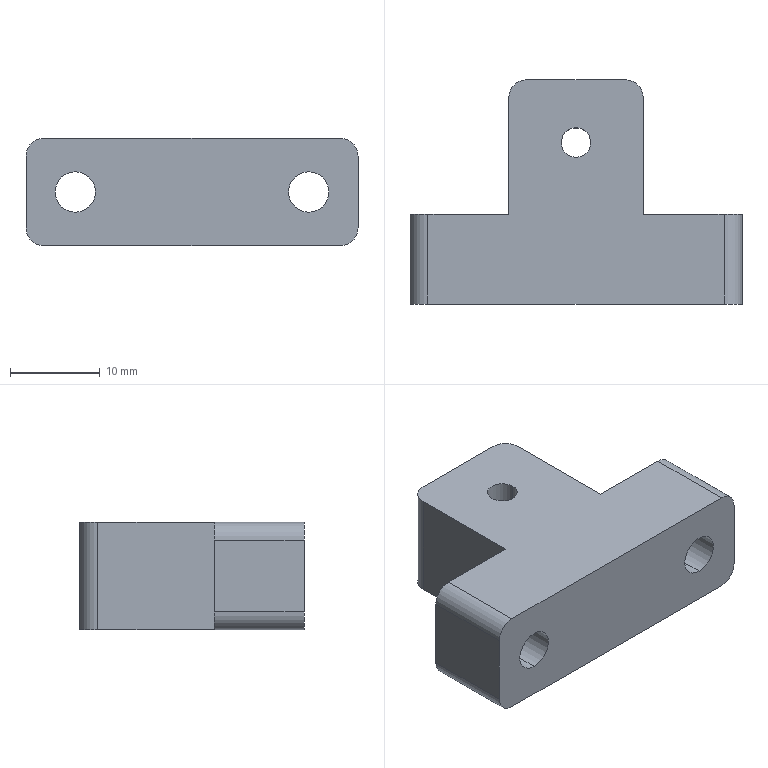Part | NX | features BREP 1 | 1 solid | 28 faces | box 37 x 25 x 12 mm | volume 6187 mm3 | cylinder 16 | plane 12 | commonest cylinder face diameters 4 x6 4.5 x4 9 x4 3.3 x2
STEP:
#1=CARTESIAN_POINT('',(7.5,23.,6.));
#2=VERTEX_POINT('',#1);
#3=CARTESIAN_POINT('',(5.5,25.,6.));
#4=VERTEX_POINT('',#3);
#5=CARTESIAN_POINT('',(5.5,23.,6.));
#6=DIRECTION('',(0.,0.,1.));
#7=DIRECTION('',(-1.,0.,0.));
#8=AXIS2_PLACEMENT_3D('',#5,#6,#7);
#9=CIRCLE('',#8,2.);
#10=EDGE_CURVE('',#2,#4,#9,.T.);
#11=ORIENTED_EDGE('',*,*,#10,.F.);
#12=CARTESIAN_POINT('',(7.5,23.,-6.));
#13=VERTEX_POINT('',#12);
#14=CARTESIAN_POINT('',(7.5,23.,6.));
#15=DIRECTION('',(0.,0.,1.));
#16=VECTOR('',#15,1000.);
#17=LINE('',#14,#16);
#18=EDGE_CURVE('',#13,#2,#17,.T.);
#19=ORIENTED_EDGE('',*,*,#18,.F.);
#20=CARTESIAN_POINT('',(5.5,25.,-6.));
#21=VERTEX_POINT('',#20);
#22=CARTESIAN_POINT('',(5.5,23.,-6.));
#23=DIRECTION('',(0.,0.,-1.));
#24=DIRECTION('',(-1.,0.,0.));
#25=AXIS2_PLACEMENT_3D('',#22,#23,#24);
#26=CIRCLE('',#25,2.);
#27=EDGE_CURVE('',#21,#13,#26,.T.);
#28=ORIENTED_EDGE('',*,*,#27,.F.);
#29=CARTESIAN_POINT('',(5.5,25.,6.));
#30=DIRECTION('',(0.,0.,-1.));
#31=VECTOR('',#30,1000.);
#32=LINE('',#29,#31);
#33=EDGE_CURVE('',#4,#21,#32,.T.);
#34=ORIENTED_EDGE('',*,*,#33,.F.);
#35=EDGE_LOOP('',(#11,#19,#28,#34));
#36=FACE_BOUND('',#35,.T.);
#37=CARTESIAN_POINT('',(5.5,23.,6.));
#38=DIRECTION('',(0.,0.,-1.));
#39=DIRECTION('',(-1.,0.,0.));
#40=AXIS2_PLACEMENT_3D('',#37,#38,#39);
#41=CYLINDRICAL_SURFACE('',#40,2.);
#42=ADVANCED_FACE('',(#36),#41,.T.);
#43=CARTESIAN_POINT('',(-5.5,25.,6.));
#44=VERTEX_POINT('',#43);
#45=CARTESIAN_POINT('',(-7.5,23.,6.));
#46=VERTEX_POINT('',#45);
#47=CARTESIAN_POINT('',(-5.5,23.,6.));
#48=DIRECTION('',(0.,0.,1.));
#49=DIRECTION('',(-1.,0.,0.));
#50=AXIS2_PLACEMENT_3D('',#47,#48,#49);
#51=CIRCLE('',#50,2.);
#52=EDGE_CURVE('',#44,#46,#51,.T.);
#53=ORIENTED_EDGE('',*,*,#52,.F.);
#54=CARTESIAN_POINT('',(-5.5,25.,-6.));
#55=VERTEX_POINT('',#54);
#56=CARTESIAN_POINT('',(-5.5,25.,6.));
#57=DIRECTION('',(0.,0.,1.));
#58=VECTOR('',#57,1000.);
#59=LINE('',#56,#58);
#60=EDGE_CURVE('',#55,#44,#59,.T.);
#61=ORIENTED_EDGE('',*,*,#60,.F.);
#62=CARTESIAN_POINT('',(-7.5,23.,-6.));
#63=VERTEX_POINT('',#62);
#64=CARTESIAN_POINT('',(-5.5,23.,-6.));
#65=DIRECTION('',(0.,0.,-1.));
#66=DIRECTION('',(-1.,0.,0.));
#67=AXIS2_PLACEMENT_3D('',#64,#65,#66);
#68=CIRCLE('',#67,2.);
#69=EDGE_CURVE('',#63,#55,#68,.T.);
#70=ORIENTED_EDGE('',*,*,#69,.F.);
#71=CARTESIAN_POINT('',(-7.5,23.,6.));
#72=DIRECTION('',(0.,0.,-1.));
#73=VECTOR('',#72,1000.);
#74=LINE('',#71,#73);
#75=EDGE_CURVE('',#46,#63,#74,.T.);
#76=ORIENTED_EDGE('',*,*,#75,.F.);
#77=EDGE_LOOP('',(#53,#61,#70,#76));
#78=FACE_BOUND('',#77,.T.);
#79=CARTESIAN_POINT('',(-5.5,23.,6.));
#80=DIRECTION('',(0.,0.,-1.));
#81=DIRECTION('',(-1.,0.,0.));
#82=AXIS2_PLACEMENT_3D('',#79,#80,#81);
#83=CYLINDRICAL_SURFACE('',#82,2.);
#84=ADVANCED_FACE('',(#78),#83,.T.);
#85=CARTESIAN_POINT('',(16.5,0.,-6.));
#86=VERTEX_POINT('',#85);
#87=CARTESIAN_POINT('',(18.5,0.,-4.));
#88=VERTEX_POINT('',#87);
#89=CARTESIAN_POINT('',(16.5,0.,-4.));
#90=DIRECTION('',(0.,-1.,0.));
#91=DIRECTION('',(0.,0.,1.));
#92=AXIS2_PLACEMENT_3D('',#89,#90,#91);
#93=CIRCLE('',#92,2.);
#94=EDGE_CURVE('',#86,#88,#93,.T.);
#95=ORIENTED_EDGE('',*,*,#94,.F.);
#96=CARTESIAN_POINT('',(16.5,10.,-6.));
#97=VERTEX_POINT('',#96);
#98=CARTESIAN_POINT('',(16.5,0.,-6.));
#99=DIRECTION('',(0.,-1.,0.));
#100=VECTOR('',#99,1000.);
#101=LINE('',#98,#100);
#102=EDGE_CURVE('',#97,#86,#101,.T.);
#103=ORIENTED_EDGE('',*,*,#102,.F.);
#104=CARTESIAN_POINT('',(18.5,10.,-4.));
#105=VERTEX_POINT('',#104);
#106=CARTESIAN_POINT('',(16.5,10.,-4.));
#107=DIRECTION('',(0.,1.,0.));
#108=DIRECTION('',(1.,0.,0.));
#109=AXIS2_PLACEMENT_3D('',#106,#107,#108);
#110=CIRCLE('',#109,2.);
#111=EDGE_CURVE('',#105,#97,#110,.T.);
#112=ORIENTED_EDGE('',*,*,#111,.F.);
#113=CARTESIAN_POINT('',(18.5,10.,-4.));
#114=DIRECTION('',(0.,1.,0.));
#115=VECTOR('',#114,1000.);
#116=LINE('',#113,#115);
#117=EDGE_CURVE('',#88,#105,#116,.T.);
#118=ORIENTED_EDGE('',*,*,#117,.F.);
#119=EDGE_LOOP('',(#95,#103,#112,#118));
#120=FACE_BOUND('',#119,.T.);
#121=CARTESIAN_POINT('',(16.5,10.,-4.));
#122=DIRECTION('',(0.,-1.,0.));
#123=DIRECTION('',(1.,0.,0.));
#124=AXIS2_PLACEMENT_3D('',#121,#122,#123);
#125=CYLINDRICAL_SURFACE('',#124,2.);
#126=ADVANCED_FACE('',(#120),#125,.T.);
#127=CARTESIAN_POINT('',(18.5,0.,4.));
#128=VERTEX_POINT('',#127);
#129=CARTESIAN_POINT('',(16.5,0.,6.));
#130=VERTEX_POINT('',#129);
#131=CARTESIAN_POINT('',(16.5,0.,4.));
#132=DIRECTION('',(0.,-1.,0.));
#133=DIRECTION('',(0.,0.,1.));
#134=AXIS2_PLACEMENT_3D('',#131,#132,#133);
#135=CIRCLE('',#134,2.);
#136=EDGE_CURVE('',#128,#130,#135,.T.);
#137=ORIENTED_EDGE('',*,*,#136,.F.);
#138=CARTESIAN_POINT('',(18.5,10.,4.));
#139=VERTEX_POINT('',#138);
#140=CARTESIAN_POINT('',(18.5,10.,4.));
#141=DIRECTION('',(0.,-1.,0.));
#142=VECTOR('',#141,1000.);
#143=LINE('',#140,#142);
#144=EDGE_CURVE('',#139,#128,#143,.T.);
#145=ORIENTED_EDGE('',*,*,#144,.F.);
#146=CARTESIAN_POINT('',(16.5,10.,6.));
#147=VERTEX_POINT('',#146);
#148=CARTESIAN_POINT('',(16.5,10.,4.));
#149=DIRECTION('',(0.,1.,0.));
#150=DIRECTION('',(1.,0.,0.));
#151=AXIS2_PLACEMENT_3D('',#148,#149,#150);
#152=CIRCLE('',#151,2.);
#153=EDGE_CURVE('',#147,#139,#152,.T.);
#154=ORIENTED_EDGE('',*,*,#153,.F.);
#155=CARTESIAN_POINT('',(16.5,0.,6.));
#156=DIRECTION('',(0.,1.,0.));
#157=VECTOR('',#156,1000.);
#158=LINE('',#155,#157);
#159=EDGE_CURVE('',#130,#147,#158,.T.);
#160=ORIENTED_EDGE('',*,*,#159,.F.);
#161=EDGE_LOOP('',(#137,#145,#154,#160));
#162=FACE_BOUND('',#161,.T.);
#163=CARTESIAN_POINT('',(16.5,0.,4.));
#164=DIRECTION('',(0.,1.,0.));
#165=DIRECTION('',(-1.,0.,0.));
#166=AXIS2_PLACEMENT_3D('',#163,#164,#165);
#167=CYLINDRICAL_SURFACE('',#166,2.);
#168=ADVANCED_FACE('',(#162),#167,.T.);
#169=CARTESIAN_POINT('',(-16.5,10.,-6.));
#170=VERTEX_POINT('',#169);
#171=CARTESIAN_POINT('',(-18.5,10.,-4.));
#172=VERTEX_POINT('',#171);
#173=CARTESIAN_POINT('',(-16.5,10.,-4.));
#174=DIRECTION('',(0.,1.,0.));
#175=DIRECTION('',(1.,0.,0.));
#176=AXIS2_PLACEMENT_3D('',#173,#174,#175);
#177=CIRCLE('',#176,2.);
#178=EDGE_CURVE('',#170,#172,#177,.T.);
#179=ORIENTED_EDGE('',*,*,#178,.F.);
#180=CARTESIAN_POINT('',(-16.5,0.,-6.));
#181=VERTEX_POINT('',#180);
#182=CARTESIAN_POINT('',(-16.5,10.,-6.));
#183=DIRECTION('',(0.,1.,0.));
#184=VECTOR('',#183,1000.);
#185=LINE('',#182,#184);
#186=EDGE_CURVE('',#181,#170,#185,.T.);
#187=ORIENTED_EDGE('',*,*,#186,.F.);
#188=CARTESIAN_POINT('',(-18.5,0.,-4.));
#189=VERTEX_POINT('',#188);
#190=CARTESIAN_POINT('',(-16.5,0.,-4.));
#191=DIRECTION('',(0.,-1.,0.));
#192=DIRECTION('',(0.,0.,1.));
#193=AXIS2_PLACEMENT_3D('',#190,#191,#192);
#194=CIRCLE('',#193,2.);
#195=EDGE_CURVE('',#189,#181,#194,.T.);
#196=ORIENTED_EDGE('',*,*,#195,.F.);
#197=CARTESIAN_POINT('',(-18.5,0.,-4.));
#198=DIRECTION('',(0.,-1.,0.));
#199=VECTOR('',#198,1000.);
#200=LINE('',#197,#199);
#201=EDGE_CURVE('',#172,#189,#200,.T.);
#202=ORIENTED_EDGE('',*,*,#201,.F.);
#203=EDGE_LOOP('',(#179,#187,#196,#202));
#204=FACE_BOUND('',#203,.T.);
#205=CARTESIAN_POINT('',(-16.5,10.,-4.));
#206=DIRECTION('',(0.,1.,0.));
#207=DIRECTION('',(-1.,0.,0.));
#208=AXIS2_PLACEMENT_3D('',#205,#206,#207);
#209=CYLINDRICAL_SURFACE('',#208,2.);
#210=ADVANCED_FACE('',(#204),#209,.T.);
#211=CARTESIAN_POINT('',(-18.5,10.,4.));
#212=VERTEX_POINT('',#211);
#213=CARTESIAN_POINT('',(-16.5,10.,6.));
#214=VERTEX_POINT('',#213);
#215=CARTESIAN_POINT('',(-16.5,10.,4.));
#216=DIRECTION('',(0.,1.,0.));
#217=DIRECTION('',(1.,0.,0.));
#218=AXIS2_PLACEMENT_3D('',#215,#216,#217);
#219=CIRCLE('',#218,2.);
#220=EDGE_CURVE('',#212,#214,#219,.T.);
#221=ORIENTED_EDGE('',*,*,#220,.F.);
#222=CARTESIAN_POINT('',(-18.5,0.,4.));
#223=VERTEX_POINT('',#222);
#224=CARTESIAN_POINT('',(-18.5,10.,4.));
#225=DIRECTION('',(0.,1.,0.));
#226=VECTOR('',#225,1000.);
#227=LINE('',#224,#226);
#228=EDGE_CURVE('',#223,#212,#227,.T.);
#229=ORIENTED_EDGE('',*,*,#228,.F.);
#230=CARTESIAN_POINT('',(-16.5,0.,6.));
#231=VERTEX_POINT('',#230);
#232=CARTESIAN_POINT('',(-16.5,0.,4.));
#233=DIRECTION('',(0.,-1.,0.));
#234=DIRECTION('',(0.,0.,1.));
#235=AXIS2_PLACEMENT_3D('',#232,#233,#234);
#236=CIRCLE('',#235,2.);
#237=EDGE_CURVE('',#231,#223,#236,.T.);
#238=ORIENTED_EDGE('',*,*,#237,.F.);
#239=CARTESIAN_POINT('',(-16.5,0.,6.));
#240=DIRECTION('',(0.,-1.,0.));
#241=VECTOR('',#240,1000.);
#242=LINE('',#239,#241);
#243=EDGE_CURVE('',#214,#231,#242,.T.);
#244=ORIENTED_EDGE('',*,*,#243,.F.);
#245=EDGE_LOOP('',(#221,#229,#238,#244));
#246=FACE_BOUND('',#245,.T.);
#247=CARTESIAN_POINT('',(-16.5,0.,4.));
#248=DIRECTION('',(0.,-1.,0.));
#249=DIRECTION('',(1.,0.,0.));
#250=AXIS2_PLACEMENT_3D('',#247,#248,#249);
#251=CYLINDRICAL_SURFACE('',#250,2.);
#252=ADVANCED_FACE('',(#246),#251,.T.);
#253=CARTESIAN_POINT('',(-1.65,18.,6.));
#254=VERTEX_POINT('',#253);
#255=CARTESIAN_POINT('',(-1.65,18.,-6.));
#256=VERTEX_POINT('',#255);
#257=CARTESIAN_POINT('',(-1.65,18.,6.));
#258=DIRECTION('',(0.,0.,1.));
#259=VECTOR('',#258,1000.);
#260=LINE('',#257,#259);
#261=EDGE_CURVE('',#254,#256,#260,.F.);
#262=ORIENTED_EDGE('',*,*,#261,.T.);
#263=CARTESIAN_POINT('',(1.65,18.,-6.));
#264=VERTEX_POINT('',#263);
#265=CARTESIAN_POINT('',(0.,18.,-6.));
#266=DIRECTION('',(0.,0.,-1.));
#267=DIRECTION('',(-1.,0.,0.));
#268=AXIS2_PLACEMENT_3D('',#265,#266,#267);
#269=CIRCLE('',#268,1.65);
#270=EDGE_CURVE('',#256,#264,#269,.T.);
#271=ORIENTED_EDGE('',*,*,#270,.T.);
#272=CARTESIAN_POINT('',(1.65,18.,6.));
#273=VERTEX_POINT('',#272);
#274=CARTESIAN_POINT('',(1.65,18.,6.));
#275=DIRECTION('',(0.,0.,1.));
#276=VECTOR('',#275,1000.);
#277=LINE('',#274,#276);
#278=EDGE_CURVE('',#273,#264,#277,.F.);
#279=ORIENTED_EDGE('',*,*,#278,.F.);
#280=CARTESIAN_POINT('',(0.,18.,6.));
#281=DIRECTION('',(0.,0.,1.));
#282=DIRECTION('',(1.,0.,0.));
#283=AXIS2_PLACEMENT_3D('',#280,#281,#282);
#284=CIRCLE('',#283,1.65);
#285=EDGE_CURVE('',#273,#254,#284,.T.);
#286=ORIENTED_EDGE('',*,*,#285,.T.);
#287=EDGE_LOOP('',(#262,#271,#279,#286));
#288=FACE_BOUND('',#287,.T.);
#289=CARTESIAN_POINT('',(0.,18.,6.));
#290=DIRECTION('',(0.,0.,1.));
#291=DIRECTION('',(1.,0.,0.));
#292=AXIS2_PLACEMENT_3D('',#289,#290,#291);
#293=CYLINDRICAL_SURFACE('',#292,1.65);
#294=ADVANCED_FACE('',(#288),#293,.F.);
#295=CARTESIAN_POINT('',(13.,10.,-4.5));
#296=VERTEX_POINT('',#295);
#297=CARTESIAN_POINT('',(13.,5.,-4.5));
#298=VERTEX_POINT('',#297);
#299=CARTESIAN_POINT('',(13.,10.,-4.5));
#300=DIRECTION('',(0.,1.,0.));
#301=VECTOR('',#300,1000.);
#302=LINE('',#299,#301);
#303=EDGE_CURVE('',#296,#298,#302,.F.);
#304=ORIENTED_EDGE('',*,*,#303,.T.);
#305=CARTESIAN_POINT('',(13.,5.,4.5));
#306=VERTEX_POINT('',#305);
#307=CARTESIAN_POINT('',(13.,5.,0.));
#308=DIRECTION('',(0.,1.,0.));
#309=DIRECTION('',(0.,0.,1.));
#310=AXIS2_PLACEMENT_3D('',#307,#308,#309);
#311=CIRCLE('',#310,4.5);
#312=EDGE_CURVE('',#306,#298,#311,.T.);
#313=ORIENTED_EDGE('',*,*,#312,.F.);
#314=CARTESIAN_POINT('',(13.,10.,4.5));
#315=VERTEX_POINT('',#314);
#316=CARTESIAN_POINT('',(13.,10.,4.5));
#317=DIRECTION('',(0.,1.,0.));
#318=VECTOR('',#317,1000.);
#319=LINE('',#316,#318);
#320=EDGE_CURVE('',#315,#306,#319,.F.);
#321=ORIENTED_EDGE('',*,*,#320,.F.);
#322=CARTESIAN_POINT('',(13.,10.,0.));
#323=DIRECTION('',(0.,1.,0.));
#324=DIRECTION('',(0.,0.,1.));
#325=AXIS2_PLACEMENT_3D('',#322,#323,#324);
#326=CIRCLE('',#325,4.5);
#327=EDGE_CURVE('',#315,#296,#326,.T.);
#328=ORIENTED_EDGE('',*,*,#327,.T.);
#329=EDGE_LOOP('',(#304,#313,#321,#328));
#330=FACE_BOUND('',#329,.T.);
#331=CARTESIAN_POINT('',(13.,10.,0.));
#332=DIRECTION('',(0.,1.,0.));
#333=DIRECTION('',(0.,0.,1.));
#334=AXIS2_PLACEMENT_3D('',#331,#332,#333);
#335=CYLINDRICAL_SURFACE('',#334,4.5);
#336=ADVANCED_FACE('',(#330),#335,.F.);
#337=ORIENTED_EDGE('',*,*,#312,.T.);
#338=CARTESIAN_POINT('',(13.,5.,0.));
#339=DIRECTION('',(0.,1.,0.));
#340=DIRECTION('',(0.,0.,1.));
#341=AXIS2_PLACEMENT_3D('',#338,#339,#340);
#342=CIRCLE('',#341,4.5);
#343=EDGE_CURVE('',#298,#306,#342,.T.);
#344=ORIENTED_EDGE('',*,*,#343,.T.);
#345=EDGE_LOOP('',(#337,#344));
#346=FACE_BOUND('',#345,.T.);
#347=CARTESIAN_POINT('',(13.,5.,2.25));
#348=VERTEX_POINT('',#347);
#349=CARTESIAN_POINT('',(13.,5.,-2.25));
#350=VERTEX_POINT('',#349);
#351=CARTESIAN_POINT('',(13.,5.,0.));
#352=DIRECTION('',(0.,1.,0.));
#353=DIRECTION('',(0.,0.,1.));
#354=AXIS2_PLACEMENT_3D('',#351,#352,#353);
#355=CIRCLE('',#354,2.25);
#356=EDGE_CURVE('',#348,#350,#355,.T.);
#357=ORIENTED_EDGE('',*,*,#356,.F.);
#358=CARTESIAN_POINT('',(13.,5.,0.));
#359=DIRECTION('',(0.,1.,0.));
#360=DIRECTION('',(0.,0.,1.));
#361=AXIS2_PLACEMENT_3D('',#358,#359,#360);
#362=CIRCLE('',#361,2.25);
#363=EDGE_CURVE('',#350,#348,#362,.T.);
#364=ORIENTED_EDGE('',*,*,#363,.F.);
#365=EDGE_LOOP('',(#357,#364));
#366=FACE_BOUND('',#365,.T.);
#367=CARTESIAN_POINT('',(15.25,5.,0.));
#368=DIRECTION('',(0.,-1.,0.));
#369=DIRECTION('',(0.,0.,-1.));
#370=AXIS2_PLACEMENT_3D('',#367,#368,#369);
#371=PLANE('',#370);
#372=ADVANCED_FACE('',(#346,#366),#371,.F.);
#373=CARTESIAN_POINT('',(13.,0.,-2.25));
#374=VERTEX_POINT('',#373);
#375=CARTESIAN_POINT('',(13.,10.,-2.25));
#376=DIRECTION('',(0.,1.,0.));
#377=VECTOR('',#376,1000.);
#378=LINE('',#375,#377);
#379=EDGE_CURVE('',#350,#374,#378,.F.);
#380=ORIENTED_EDGE('',*,*,#379,.T.);
#381=CARTESIAN_POINT('',(13.,0.,2.25));
#382=VERTEX_POINT('',#381);
#383=CARTESIAN_POINT('',(13.,0.,0.));
#384=DIRECTION('',(0.,1.,0.));
#385=DIRECTION('',(0.,0.,1.));
#386=AXIS2_PLACEMENT_3D('',#383,#384,#385);
#387=CIRCLE('',#386,2.25);
#388=EDGE_CURVE('',#382,#374,#387,.T.);
#389=ORIENTED_EDGE('',*,*,#388,.F.);
#390=CARTESIAN_POINT('',(13.,10.,2.25));
#391=DIRECTION('',(0.,1.,0.));
#392=VECTOR('',#391,1000.);
#393=LINE('',#390,#392);
#394=EDGE_CURVE('',#348,#382,#393,.F.);
#395=ORIENTED_EDGE('',*,*,#394,.F.);
#396=ORIENTED_EDGE('',*,*,#356,.T.);
#397=EDGE_LOOP('',(#380,#389,#395,#396));
#398=FACE_BOUND('',#397,.T.);
#399=CARTESIAN_POINT('',(13.,10.,0.));
#400=DIRECTION('',(0.,1.,0.));
#401=DIRECTION('',(0.,0.,1.));
#402=AXIS2_PLACEMENT_3D('',#399,#400,#401);
#403=CYLINDRICAL_SURFACE('',#402,2.25);
#404=ADVANCED_FACE('',(#398),#403,.F.);
#405=CARTESIAN_POINT('',(-13.,10.,-4.5));
#406=VERTEX_POINT('',#405);
#407=CARTESIAN_POINT('',(-13.,5.,-4.5));
#408=VERTEX_POINT('',#407);
#409=CARTESIAN_POINT('',(-13.,10.,-4.5));
#410=DIRECTION('',(0.,1.,0.));
#411=VECTOR('',#410,1000.);
#412=LINE('',#409,#411);
#413=EDGE_CURVE('',#406,#408,#412,.F.);
#414=ORIENTED_EDGE('',*,*,#413,.T.);
#415=CARTESIAN_POINT('',(-13.,5.,4.5));
#416=VERTEX_POINT('',#415);
#417=CARTESIAN_POINT('',(-13.,5.,0.));
#418=DIRECTION('',(0.,1.,0.));
#419=DIRECTION('',(0.,0.,1.));
#420=AXIS2_PLACEMENT_3D('',#417,#418,#419);
#421=CIRCLE('',#420,4.5);
#422=EDGE_CURVE('',#416,#408,#421,.T.);
#423=ORIENTED_EDGE('',*,*,#422,.F.);
#424=CARTESIAN_POINT('',(-13.,10.,4.5));
#425=VERTEX_POINT('',#424);
#426=CARTESIAN_POINT('',(-13.,10.,4.5));
#427=DIRECTION('',(0.,1.,0.));
#428=VECTOR('',#427,1000.);
#429=LINE('',#426,#428);
#430=EDGE_CURVE('',#425,#416,#429,.F.);
#431=ORIENTED_EDGE('',*,*,#430,.F.);
#432=CARTESIAN_POINT('',(-13.,10.,0.));
#433=DIRECTION('',(0.,1.,0.));
#434=DIRECTION('',(0.,0.,1.));
#435=AXIS2_PLACEMENT_3D('',#432,#433,#434);
#436=CIRCLE('',#435,4.5);
#437=EDGE_CURVE('',#425,#406,#436,.T.);
#438=ORIENTED_EDGE('',*,*,#437,.T.);
#439=EDGE_LOOP('',(#414,#423,#431,#438));
#440=FACE_BOUND('',#439,.T.);
#441=CARTESIAN_POINT('',(-13.,10.,0.));
#442=DIRECTION('',(0.,1.,0.));
#443=DIRECTION('',(0.,0.,1.));
#444=AXIS2_PLACEMENT_3D('',#441,#442,#443);
#445=CYLINDRICAL_SURFACE('',#444,4.5);
#446=ADVANCED_FACE('',(#440),#445,.F.);
#447=ORIENTED_EDGE('',*,*,#422,.T.);
#448=CARTESIAN_POINT('',(-13.,5.,0.));
#449=DIRECTION('',(0.,1.,0.));
#450=DIRECTION('',(0.,0.,1.));
#451=AXIS2_PLACEMENT_3D('',#448,#449,#450);
#452=CIRCLE('',#451,4.5);
#453=EDGE_CURVE('',#408,#416,#452,.T.);
#454=ORIENTED_EDGE('',*,*,#453,.T.);
#455=EDGE_LOOP('',(#447,#454));
#456=FACE_BOUND('',#455,.T.);
#457=CARTESIAN_POINT('',(-13.,5.,2.25));
#458=VERTEX_POINT('',#457);
#459=CARTESIAN_POINT('',(-13.,5.,-2.25));
#460=VERTEX_POINT('',#459);
#461=CARTESIAN_POINT('',(-13.,5.,0.));
#462=DIRECTION('',(0.,1.,0.));
#463=DIRECTION('',(0.,0.,1.));
#464=AXIS2_PLACEMENT_3D('',#461,#462,#463);
#465=CIRCLE('',#464,2.25);
#466=EDGE_CURVE('',#458,#460,#465,.T.);
#467=ORIENTED_EDGE('',*,*,#466,.F.);
#468=CARTESIAN_POINT('',(-13.,5.,0.));
#469=DIRECTION('',(0.,1.,0.));
#470=DIRECTION('',(0.,0.,1.));
#471=AXIS2_PLACEMENT_3D('',#468,#469,#470);
#472=CIRCLE('',#471,2.25);
#473=EDGE_CURVE('',#460,#458,#472,.T.);
#474=ORIENTED_EDGE('',*,*,#473,.F.);
#475=EDGE_LOOP('',(#467,#474));
#476=FACE_BOUND('',#475,.T.);
#477=CARTESIAN_POINT('',(-10.75,5.,0.));
#478=DIRECTION('',(0.,-1.,0.));
#479=DIRECTION('',(0.,0.,-1.));
#480=AXIS2_PLACEMENT_3D('',#477,#478,#479);
#481=PLANE('',#480);
#482=ADVANCED_FACE('',(#456,#476),#481,.F.);
#483=CARTESIAN_POINT('',(-13.,0.,-2.25));
#484=VERTEX_POINT('',#483);
#485=CARTESIAN_POINT('',(-13.,10.,-2.25));
#486=DIRECTION('',(0.,1.,0.));
#487=VECTOR('',#486,1000.);
#488=LINE('',#485,#487);
#489=EDGE_CURVE('',#460,#484,#488,.F.);
#490=ORIENTED_EDGE('',*,*,#489,.T.);
#491=CARTESIAN_POINT('',(-13.,0.,2.25));
#492=VERTEX_POINT('',#491);
#493=CARTESIAN_POINT('',(-13.,0.,0.));
#494=DIRECTION('',(0.,1.,0.));
#495=DIRECTION('',(0.,0.,1.));
#496=AXIS2_PLACEMENT_3D('',#493,#494,#495);
#497=CIRCLE('',#496,2.25);
#498=EDGE_CURVE('',#492,#484,#497,.T.);
#499=ORIENTED_EDGE('',*,*,#498,.F.);
#500=CARTESIAN_POINT('',(-13.,10.,2.25));
#501=DIRECTION('',(0.,1.,0.));
#502=VECTOR('',#501,1000.);
#503=LINE('',#500,#502);
#504=EDGE_CURVE('',#458,#492,#503,.F.);
#505=ORIENTED_EDGE('',*,*,#504,.F.);
#506=ORIENTED_EDGE('',*,*,#466,.T.);
#507=EDGE_LOOP('',(#490,#499,#505,#506));
#508=FACE_BOUND('',#507,.T.);
#509=CARTESIAN_POINT('',(-13.,10.,0.));
#510=DIRECTION('',(0.,1.,0.));
#511=DIRECTION('',(0.,0.,1.));
#512=AXIS2_PLACEMENT_3D('',#509,#510,#511);
#513=CYLINDRICAL_SURFACE('',#512,2.25);
#514=ADVANCED_FACE('',(#508),#513,.F.);
#515=CARTESIAN_POINT('',(-18.5,0.,-6.));
#516=DIRECTION('',(1.,0.,0.));
#517=VECTOR('',#516,1000.);
#518=LINE('',#515,#517);
#519=EDGE_CURVE('',#181,#86,#518,.T.);
#520=ORIENTED_EDGE('',*,*,#519,.F.);
#521=ORIENTED_EDGE('',*,*,#186,.T.);
#522=CARTESIAN_POINT('',(-7.5,10.,-6.));
#523=VERTEX_POINT('',#522);
#524=CARTESIAN_POINT('',(-7.5,10.,-6.));
#525=DIRECTION('',(-1.,0.,0.));
#526=VECTOR('',#525,1000.);
#527=LINE('',#524,#526);
#528=EDGE_CURVE('',#523,#170,#527,.T.);
#529=ORIENTED_EDGE('',*,*,#528,.F.);
#530=CARTESIAN_POINT('',(-7.5,25.,-6.));
#531=DIRECTION('',(0.,-1.,0.));
#532=VECTOR('',#531,1000.);
#533=LINE('',#530,#532);
#534=EDGE_CURVE('',#63,#523,#533,.T.);
#535=ORIENTED_EDGE('',*,*,#534,.F.);
#536=ORIENTED_EDGE('',*,*,#69,.T.);
#537=CARTESIAN_POINT('',(7.5,25.,-6.));
#538=DIRECTION('',(-1.,0.,0.));
#539=VECTOR('',#538,1000.);
#540=LINE('',#537,#539);
#541=EDGE_CURVE('',#21,#55,#540,.T.);
#542=ORIENTED_EDGE('',*,*,#541,.F.);
#543=ORIENTED_EDGE('',*,*,#27,.T.);
#544=CARTESIAN_POINT('',(7.5,10.,-6.));
#545=VERTEX_POINT('',#544);
#546=CARTESIAN_POINT('',(7.5,25.,-6.));
#547=DIRECTION('',(0.,1.,0.));
#548=VECTOR('',#547,1000.);
#549=LINE('',#546,#548);
#550=EDGE_CURVE('',#545,#13,#549,.T.);
#551=ORIENTED_EDGE('',*,*,#550,.F.);
#552=CARTESIAN_POINT('',(7.5,10.,-6.));
#553=DIRECTION('',(-1.,0.,0.));
#554=VECTOR('',#553,1000.);
#555=LINE('',#552,#554);
#556=EDGE_CURVE('',#97,#545,#555,.T.);
#557=ORIENTED_EDGE('',*,*,#556,.F.);
#558=ORIENTED_EDGE('',*,*,#102,.T.);
#559=EDGE_LOOP('',(#520,#521,#529,#535,#536,#542,#543,#551,#557,#558));
#560=FACE_BOUND('',#559,.T.);
#561=CARTESIAN_POINT('',(0.,18.,-6.));
#562=DIRECTION('',(0.,0.,-1.));
#563=DIRECTION('',(-1.,0.,0.));
#564=AXIS2_PLACEMENT_3D('',#561,#562,#563);
#565=CIRCLE('',#564,1.65);
#566=EDGE_CURVE('',#264,#256,#565,.T.);
#567=ORIENTED_EDGE('',*,*,#566,.F.);
#568=ORIENTED_EDGE('',*,*,#270,.F.);
#569=EDGE_LOOP('',(#567,#568));
#570=FACE_BOUND('',#569,.T.);
#571=CARTESIAN_POINT('',(0.,0.,-6.));
#572=DIRECTION('',(0.,0.,-1.));
#573=DIRECTION('',(-1.,0.,0.));
#574=AXIS2_PLACEMENT_3D('',#571,#572,#573);
#575=PLANE('',#574);
#576=ADVANCED_FACE('',(#560,#570),#575,.T.);
#577=CARTESIAN_POINT('',(-7.5,10.,6.));
#578=VERTEX_POINT('',#577);
#579=CARTESIAN_POINT('',(-7.5,10.,6.));
#580=DIRECTION('',(-1.,0.,0.));
#581=VECTOR('',#580,1000.);
#582=LINE('',#579,#581);
#583=EDGE_CURVE('',#578,#214,#582,.T.);
#584=ORIENTED_EDGE('',*,*,#583,.T.);
#585=ORIENTED_EDGE('',*,*,#243,.T.);
#586=CARTESIAN_POINT('',(-18.5,0.,6.));
#587=DIRECTION('',(1.,0.,0.));
#588=VECTOR('',#587,1000.);
#589=LINE('',#586,#588);
#590=EDGE_CURVE('',#231,#130,#589,.T.);
#591=ORIENTED_EDGE('',*,*,#590,.T.);
#592=ORIENTED_EDGE('',*,*,#159,.T.);
#593=CARTESIAN_POINT('',(7.5,10.,6.));
#594=VERTEX_POINT('',#593);
#595=CARTESIAN_POINT('',(7.5,10.,6.));
#596=DIRECTION('',(-1.,0.,0.));
#597=VECTOR('',#596,1000.);
#598=LINE('',#595,#597);
#599=EDGE_CURVE('',#147,#594,#598,.T.);
#600=ORIENTED_EDGE('',*,*,#599,.T.);
#601=CARTESIAN_POINT('',(7.5,25.,6.));
#602=DIRECTION('',(0.,1.,0.));
#603=VECTOR('',#602,1000.);
#604=LINE('',#601,#603);
#605=EDGE_CURVE('',#594,#2,#604,.T.);
#606=ORIENTED_EDGE('',*,*,#605,.T.);
#607=ORIENTED_EDGE('',*,*,#10,.T.);
#608=CARTESIAN_POINT('',(7.5,25.,6.));
#609=DIRECTION('',(-1.,0.,0.));
#610=VECTOR('',#609,1000.);
#611=LINE('',#608,#610);
#612=EDGE_CURVE('',#4,#44,#611,.T.);
#613=ORIENTED_EDGE('',*,*,#612,.T.);
#614=ORIENTED_EDGE('',*,*,#52,.T.);
#615=CARTESIAN_POINT('',(-7.5,25.,6.));
#616=DIRECTION('',(0.,-1.,0.));
#617=VECTOR('',#616,1000.);
#618=LINE('',#615,#617);
#619=EDGE_CURVE('',#46,#578,#618,.T.);
#620=ORIENTED_EDGE('',*,*,#619,.T.);
#621=EDGE_LOOP('',(#584,#585,#591,#592,#600,#606,#607,#613,#614,#620));
#622=FACE_BOUND('',#621,.T.);
#623=ORIENTED_EDGE('',*,*,#285,.F.);
#624=CARTESIAN_POINT('',(0.,18.,6.));
#625=DIRECTION('',(0.,0.,1.));
#626=DIRECTION('',(1.,0.,0.));
#627=AXIS2_PLACEMENT_3D('',#624,#625,#626);
#628=CIRCLE('',#627,1.65);
#629=EDGE_CURVE('',#254,#273,#628,.T.);
#630=ORIENTED_EDGE('',*,*,#629,.F.);
#631=EDGE_LOOP('',(#623,#630));
#632=FACE_BOUND('',#631,.T.);
#633=CARTESIAN_POINT('',(0.,0.,6.));
#634=DIRECTION('',(0.,0.,-1.));
#635=DIRECTION('',(-1.,0.,0.));
#636=AXIS2_PLACEMENT_3D('',#633,#634,#635);
#637=PLANE('',#636);
#638=ADVANCED_FACE('',(#622,#632),#637,.F.);
#639=ORIENTED_EDGE('',*,*,#541,.T.);
#640=ORIENTED_EDGE('',*,*,#60,.T.);
#641=ORIENTED_EDGE('',*,*,#612,.F.);
#642=ORIENTED_EDGE('',*,*,#33,.T.);
#643=EDGE_LOOP('',(#639,#640,#641,#642));
#644=FACE_BOUND('',#643,.T.);
#645=CARTESIAN_POINT('',(7.5,25.,6.));
#646=DIRECTION('',(0.,-1.,0.));
#647=DIRECTION('',(0.,0.,-1.));
#648=AXIS2_PLACEMENT_3D('',#645,#646,#647);
#649=PLANE('',#648);
#650=ADVANCED_FACE('',(#644),#649,.F.);
#651=ORIENTED_EDGE('',*,*,#550,.T.);
#652=ORIENTED_EDGE('',*,*,#18,.T.);
#653=ORIENTED_EDGE('',*,*,#605,.F.);
#654=CARTESIAN_POINT('',(7.5,10.,6.));
#655=DIRECTION('',(0.,0.,-1.));
#656=VECTOR('',#655,1000.);
#657=LINE('',#654,#656);
#658=EDGE_CURVE('',#594,#545,#657,.T.);
#659=ORIENTED_EDGE('',*,*,#658,.T.);
#660=EDGE_LOOP('',(#651,#652,#653,#659));
#661=FACE_BOUND('',#660,.T.);
#662=CARTESIAN_POINT('',(7.5,25.,6.));
#663=DIRECTION('',(-1.,0.,0.));
#664=DIRECTION('',(0.,-1.,0.));
#665=AXIS2_PLACEMENT_3D('',#662,#663,#664);
#666=PLANE('',#665);
#667=ADVANCED_FACE('',(#661),#666,.F.);
#668=CARTESIAN_POINT('',(18.5,10.,6.));
#669=DIRECTION('',(0.,0.,-1.));
#670=VECTOR('',#669,1000.);
#671=LINE('',#668,#670);
#672=EDGE_CURVE('',#139,#105,#671,.T.);
#673=ORIENTED_EDGE('',*,*,#672,.F.);
#674=ORIENTED_EDGE('',*,*,#144,.T.);
#675=CARTESIAN_POINT('',(18.5,0.,6.));
#676=DIRECTION('',(0.,0.,-1.));
#677=VECTOR('',#676,1000.);
#678=LINE('',#675,#677);
#679=EDGE_CURVE('',#128,#88,#678,.T.);
#680=ORIENTED_EDGE('',*,*,#679,.T.);
#681=ORIENTED_EDGE('',*,*,#117,.T.);
#682=EDGE_LOOP('',(#673,#674,#680,#681));
#683=FACE_BOUND('',#682,.T.);
#684=CARTESIAN_POINT('',(18.5,10.,6.));
#685=DIRECTION('',(-1.,0.,0.));
#686=DIRECTION('',(0.,-1.,0.));
#687=AXIS2_PLACEMENT_3D('',#684,#685,#686);
#688=PLANE('',#687);
#689=ADVANCED_FACE('',(#683),#688,.F.);
#690=ORIENTED_EDGE('',*,*,#590,.F.);
#691=ORIENTED_EDGE('',*,*,#237,.T.);
#692=CARTESIAN_POINT('',(-18.5,0.,6.));
#693=DIRECTION('',(0.,0.,-1.));
#694=VECTOR('',#693,1000.);
#695=LINE('',#692,#694);
#696=EDGE_CURVE('',#223,#189,#695,.T.);
#697=ORIENTED_EDGE('',*,*,#696,.T.);
#698=ORIENTED_EDGE('',*,*,#195,.T.);
#699=ORIENTED_EDGE('',*,*,#519,.T.);
#700=ORIENTED_EDGE('',*,*,#94,.T.);
#701=ORIENTED_EDGE('',*,*,#679,.F.);
#702=ORIENTED_EDGE('',*,*,#136,.T.);
#703=EDGE_LOOP('',(#690,#691,#697,#698,#699,#700,#701,#702));
#704=FACE_BOUND('',#703,.T.);
#705=ORIENTED_EDGE('',*,*,#498,.T.);
#706=CARTESIAN_POINT('',(-13.,0.,0.));
#707=DIRECTION('',(0.,1.,0.));
#708=DIRECTION('',(0.,0.,1.));
#709=AXIS2_PLACEMENT_3D('',#706,#707,#708);
#710=CIRCLE('',#709,2.25);
#711=EDGE_CURVE('',#484,#492,#710,.T.);
#712=ORIENTED_EDGE('',*,*,#711,.T.);
#713=EDGE_LOOP('',(#705,#712));
#714=FACE_BOUND('',#713,.T.);
#715=ORIENTED_EDGE('',*,*,#388,.T.);
#716=CARTESIAN_POINT('',(13.,0.,0.));
#717=DIRECTION('',(0.,1.,0.));
#718=DIRECTION('',(0.,0.,1.));
#719=AXIS2_PLACEMENT_3D('',#716,#717,#718);
#720=CIRCLE('',#719,2.25);
#721=EDGE_CURVE('',#374,#382,#720,.T.);
#722=ORIENTED_EDGE('',*,*,#721,.T.);
#723=EDGE_LOOP('',(#715,#722));
#724=FACE_BOUND('',#723,.T.);
#725=CARTESIAN_POINT('',(-18.5,0.,6.));
#726=DIRECTION('',(0.,1.,0.));
#727=DIRECTION('',(0.,0.,1.));
#728=AXIS2_PLACEMENT_3D('',#725,#726,#727);
#729=PLANE('',#728);
#730=ADVANCED_FACE('',(#704,#714,#724),#729,.F.);
#731=ORIENTED_EDGE('',*,*,#696,.F.);
#732=ORIENTED_EDGE('',*,*,#228,.T.);
#733=CARTESIAN_POINT('',(-18.5,10.,6.));
#734=DIRECTION('',(0.,0.,-1.));
#735=VECTOR('',#734,1000.);
#736=LINE('',#733,#735);
#737=EDGE_CURVE('',#212,#172,#736,.T.);
#738=ORIENTED_EDGE('',*,*,#737,.T.);
#739=ORIENTED_EDGE('',*,*,#201,.T.);
#740=EDGE_LOOP('',(#731,#732,#738,#739));
#741=FACE_BOUND('',#740,.T.);
#742=CARTESIAN_POINT('',(-18.5,10.,6.));
#743=DIRECTION('',(1.,0.,0.));
#744=DIRECTION('',(0.,1.,0.));
#745=AXIS2_PLACEMENT_3D('',#742,#743,#744);
#746=PLANE('',#745);
#747=ADVANCED_FACE('',(#741),#746,.F.);
#748=ORIENTED_EDGE('',*,*,#737,.F.);
#749=ORIENTED_EDGE('',*,*,#220,.T.);
#750=ORIENTED_EDGE('',*,*,#583,.F.);
#751=CARTESIAN_POINT('',(-7.5,10.,6.));
#752=DIRECTION('',(0.,0.,-1.));
#753=VECTOR('',#752,1000.);
#754=LINE('',#751,#753);
#755=EDGE_CURVE('',#578,#523,#754,.T.);
#756=ORIENTED_EDGE('',*,*,#755,.T.);
#757=ORIENTED_EDGE('',*,*,#528,.T.);
#758=ORIENTED_EDGE('',*,*,#178,.T.);
#759=EDGE_LOOP('',(#748,#749,#750,#756,#757,#758));
#760=FACE_BOUND('',#759,.T.);
#761=ORIENTED_EDGE('',*,*,#437,.F.);
#762=CARTESIAN_POINT('',(-13.,10.,0.));
#763=DIRECTION('',(0.,1.,0.));
#764=DIRECTION('',(0.,0.,1.));
#765=AXIS2_PLACEMENT_3D('',#762,#763,#764);
#766=CIRCLE('',#765,4.5);
#767=EDGE_CURVE('',#406,#425,#766,.T.);
#768=ORIENTED_EDGE('',*,*,#767,.F.);
#769=EDGE_LOOP('',(#761,#768));
#770=FACE_BOUND('',#769,.T.);
#771=CARTESIAN_POINT('',(-7.5,10.,6.));
#772=DIRECTION('',(0.,-1.,0.));
#773=DIRECTION('',(1.,0.,0.));
#774=AXIS2_PLACEMENT_3D('',#771,#772,#773);
#775=PLANE('',#774);
#776=ADVANCED_FACE('',(#760,#770),#775,.F.);
#777=ORIENTED_EDGE('',*,*,#619,.F.);
#778=ORIENTED_EDGE('',*,*,#75,.T.);
#779=ORIENTED_EDGE('',*,*,#534,.T.);
#780=ORIENTED_EDGE('',*,*,#755,.F.);
#781=EDGE_LOOP('',(#777,#778,#779,#780));
#782=FACE_BOUND('',#781,.T.);
#783=CARTESIAN_POINT('',(-7.5,25.,6.));
#784=DIRECTION('',(1.,0.,0.));
#785=DIRECTION('',(0.,1.,0.));
#786=AXIS2_PLACEMENT_3D('',#783,#784,#785);
#787=PLANE('',#786);
#788=ADVANCED_FACE('',(#782),#787,.F.);
#789=ORIENTED_EDGE('',*,*,#327,.F.);
#790=CARTESIAN_POINT('',(13.,10.,0.));
#791=DIRECTION('',(0.,1.,0.));
#792=DIRECTION('',(0.,0.,1.));
#793=AXIS2_PLACEMENT_3D('',#790,#791,#792);
#794=CIRCLE('',#793,4.5);
#795=EDGE_CURVE('',#296,#315,#794,.T.);
#796=ORIENTED_EDGE('',*,*,#795,.F.);
#797=EDGE_LOOP('',(#789,#796));
#798=FACE_BOUND('',#797,.T.);
#799=ORIENTED_EDGE('',*,*,#599,.F.);
#800=ORIENTED_EDGE('',*,*,#153,.T.);
#801=ORIENTED_EDGE('',*,*,#672,.T.);
#802=ORIENTED_EDGE('',*,*,#111,.T.);
#803=ORIENTED_EDGE('',*,*,#556,.T.);
#804=ORIENTED_EDGE('',*,*,#658,.F.);
#805=EDGE_LOOP('',(#799,#800,#801,#802,#803,#804));
#806=FACE_BOUND('',#805,.T.);
#807=CARTESIAN_POINT('',(7.5,10.,6.));
#808=DIRECTION('',(0.,-1.,0.));
#809=DIRECTION('',(1.,0.,0.));
#810=AXIS2_PLACEMENT_3D('',#807,#808,#809);
#811=PLANE('',#810);
#812=ADVANCED_FACE('',(#798,#806),#811,.F.);
#813=ORIENTED_EDGE('',*,*,#711,.F.);
#814=ORIENTED_EDGE('',*,*,#489,.F.);
#815=ORIENTED_EDGE('',*,*,#473,.T.);
#816=ORIENTED_EDGE('',*,*,#504,.T.);
#817=EDGE_LOOP('',(#813,#814,#815,#816));
#818=FACE_BOUND('',#817,.T.);
#819=CARTESIAN_POINT('',(-13.,10.,0.));
#820=DIRECTION('',(0.,1.,0.));
#821=DIRECTION('',(0.,0.,1.));
#822=AXIS2_PLACEMENT_3D('',#819,#820,#821);
#823=CYLINDRICAL_SURFACE('',#822,2.25);
#824=ADVANCED_FACE('',(#818),#823,.F.);
#825=ORIENTED_EDGE('',*,*,#453,.F.);
#826=ORIENTED_EDGE('',*,*,#413,.F.);
#827=ORIENTED_EDGE('',*,*,#767,.T.);
#828=ORIENTED_EDGE('',*,*,#430,.T.);
#829=EDGE_LOOP('',(#825,#826,#827,#828));
#830=FACE_BOUND('',#829,.T.);
#831=CARTESIAN_POINT('',(-13.,10.,0.));
#832=DIRECTION('',(0.,1.,0.));
#833=DIRECTION('',(0.,0.,1.));
#834=AXIS2_PLACEMENT_3D('',#831,#832,#833);
#835=CYLINDRICAL_SURFACE('',#834,4.5);
#836=ADVANCED_FACE('',(#830),#835,.F.);
#837=ORIENTED_EDGE('',*,*,#721,.F.);
#838=ORIENTED_EDGE('',*,*,#379,.F.);
#839=ORIENTED_EDGE('',*,*,#363,.T.);
#840=ORIENTED_EDGE('',*,*,#394,.T.);
#841=EDGE_LOOP('',(#837,#838,#839,#840));
#842=FACE_BOUND('',#841,.T.);
#843=CARTESIAN_POINT('',(13.,10.,0.));
#844=DIRECTION('',(0.,1.,0.));
#845=DIRECTION('',(0.,0.,1.));
#846=AXIS2_PLACEMENT_3D('',#843,#844,#845);
#847=CYLINDRICAL_SURFACE('',#846,2.25);
#848=ADVANCED_FACE('',(#842),#847,.F.);
#849=ORIENTED_EDGE('',*,*,#343,.F.);
#850=ORIENTED_EDGE('',*,*,#303,.F.);
#851=ORIENTED_EDGE('',*,*,#795,.T.);
#852=ORIENTED_EDGE('',*,*,#320,.T.);
#853=EDGE_LOOP('',(#849,#850,#851,#852));
#854=FACE_BOUND('',#853,.T.);
#855=CARTESIAN_POINT('',(13.,10.,0.));
#856=DIRECTION('',(0.,1.,0.));
#857=DIRECTION('',(0.,0.,1.));
#858=AXIS2_PLACEMENT_3D('',#855,#856,#857);
#859=CYLINDRICAL_SURFACE('',#858,4.5);
#860=ADVANCED_FACE('',(#854),#859,.F.);
#861=ORIENTED_EDGE('',*,*,#566,.T.);
#862=ORIENTED_EDGE('',*,*,#261,.F.);
#863=ORIENTED_EDGE('',*,*,#629,.T.);
#864=ORIENTED_EDGE('',*,*,#278,.T.);
#865=EDGE_LOOP('',(#861,#862,#863,#864));
#866=FACE_BOUND('',#865,.T.);
#867=CARTESIAN_POINT('',(0.,18.,6.));
#868=DIRECTION('',(0.,0.,1.));
#869=DIRECTION('',(1.,0.,0.));
#870=AXIS2_PLACEMENT_3D('',#867,#868,#869);
#871=CYLINDRICAL_SURFACE('',#870,1.65);
#872=ADVANCED_FACE('',(#866),#871,.F.);
#873=CLOSED_SHELL('',(#42,#84,#126,#168,#210,#252,#294,#336,#372,#404,#446,#482,#514,#576,#638,#650,#667,#689,#730,#747,#776,#788,#812,#824,#836,#848,#860,#872));
#874=MANIFOLD_SOLID_BREP('',#873);
#875=(LENGTH_UNIT()NAMED_UNIT(*)SI_UNIT(.MILLI.,.METRE.));
#876=UNCERTAINTY_MEASURE_WITH_UNIT(LENGTH_MEASURE(0.00001),#875,'','');
#877=(NAMED_UNIT(*)PLANE_ANGLE_UNIT()SI_UNIT($,.RADIAN.));
#878=(NAMED_UNIT(*)SI_UNIT($,.STERADIAN.)SOLID_ANGLE_UNIT());
#879=(GEOMETRIC_REPRESENTATION_CONTEXT(3)GLOBAL_UNCERTAINTY_ASSIGNED_CONTEXT((#876))GLOBAL_UNIT_ASSIGNED_CONTEXT((#875,#877,#878))REPRESENTATION_CONTEXT('',''));
#880=ADVANCED_BREP_SHAPE_REPRESENTATION('',(#874),#879);